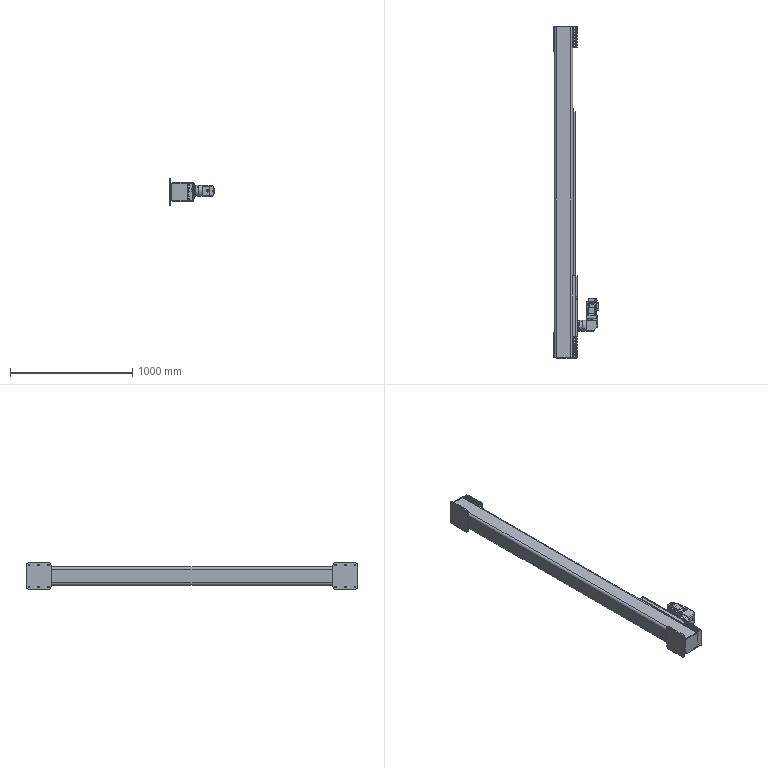Part | SolidWorks | features ReferencePattern 5, LocalLPattern 2, MirrorCompFeat 2 | 38 solids | 9099 faces | volume 18104640 mm3 | plane 5919 | cylinder 1694 | spline 1144 | torus 142 | sphere 118 | cone 82 | commonest cylinder face diameters 4.5 x196 5.2 x180 7.5 x136 1 x116 4 x78 3.3 x76